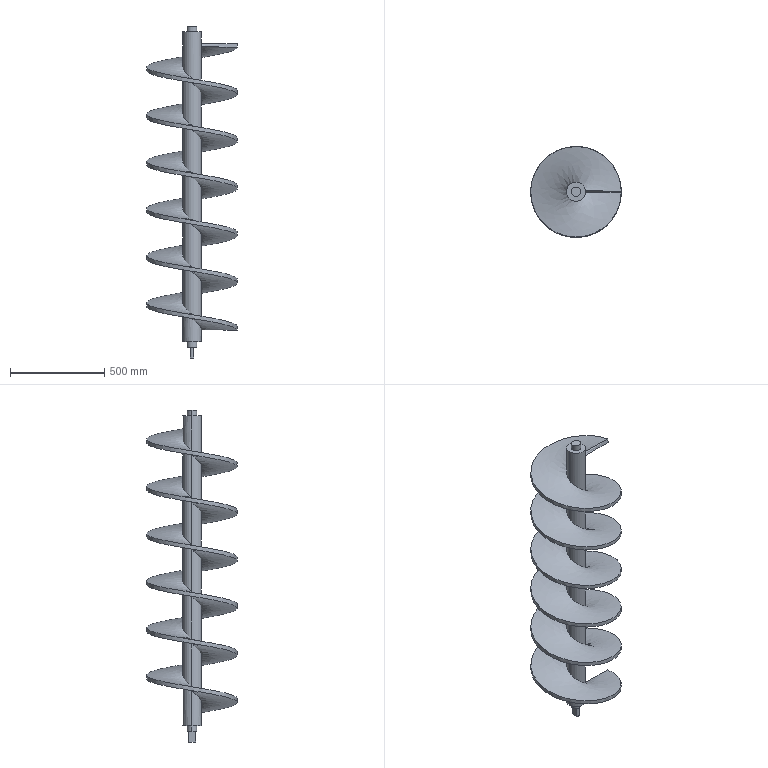Part | SolidWorks | 1 solid | 32 faces | box 480.011 x 480.011 x 1760 mm | volume 34687851 mm3 | cylinder 20 | plane 7 | spline 5 | commonest cylinder face diameters 100 x14 50 x4 40 x2